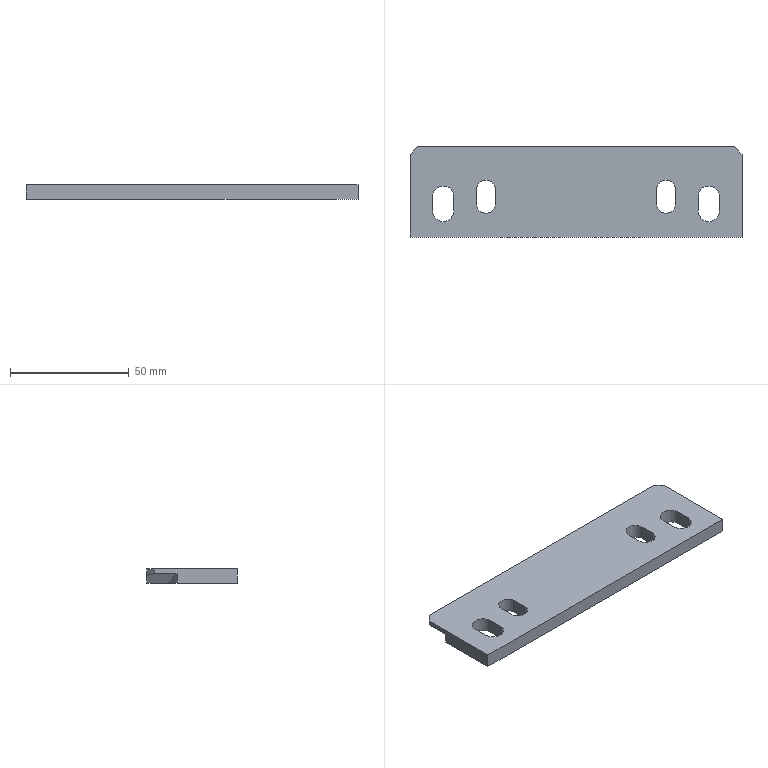Part | STEP file | gslz 2016.10.28-13_id734_x_t | 1 solid | 29 faces | box 140 x 38 x 6 mm | volume 28803 mm3 | plane 21 | cylinder 8 | commonest cylinder face diameters 8 x4 9 x4